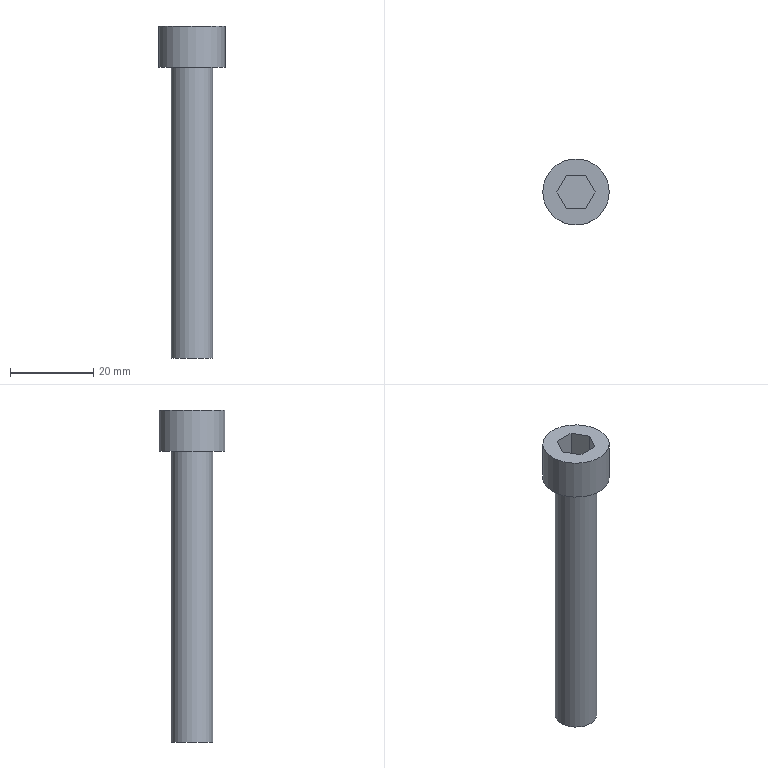Part | STEP file | 冲床-300配套压波_id14_x_t | 1 solid | 12 faces | box 16 x 16 x 80 mm | volume 7143 mm3 | plane 10 | cylinder 2 | commonest cylinder face diameters 10 x1 16 x1
STEP:
#1=CARTESIAN_POINT('',(1193.,0.,-1.));
#2=VERTEX_POINT('',#1);
#3=CARTESIAN_POINT('',(1185.,0.,-1.));
#4=DIRECTION('',(0.,0.,1.));
#5=DIRECTION('',(1.,0.,0.));
#6=AXIS2_PLACEMENT_3D('',#3,#4,#5);
#7=CIRCLE('',#6,8.);
#8=EDGE_CURVE('',#2,#2,#7,.T.);
#9=ORIENTED_EDGE('',*,*,#8,.T.);
#10=EDGE_LOOP('',(#9));
#11=FACE_BOUND('',#10,.T.);
#12=CARTESIAN_POINT('',(1182.691,4.,-1.));
#13=VERTEX_POINT('',#12);
#14=CARTESIAN_POINT('',(1187.309,4.,-1.));
#15=VERTEX_POINT('',#14);
#16=CARTESIAN_POINT('',(1182.691,4.,-1.));
#17=DIRECTION('',(1.,0.,0.));
#18=VECTOR('',#17,1.);
#19=LINE('',#16,#18);
#20=EDGE_CURVE('',#13,#15,#19,.T.);
#21=ORIENTED_EDGE('',*,*,#20,.T.);
#22=CARTESIAN_POINT('',(1189.619,0.,-1.));
#23=VERTEX_POINT('',#22);
#24=CARTESIAN_POINT('',(1187.309,4.,-1.));
#25=DIRECTION('',(0.5,-0.866,0.));
#26=VECTOR('',#25,1.);
#27=LINE('',#24,#26);
#28=EDGE_CURVE('',#15,#23,#27,.T.);
#29=ORIENTED_EDGE('',*,*,#28,.T.);
#30=CARTESIAN_POINT('',(1187.309,-4.,-1.));
#31=VERTEX_POINT('',#30);
#32=CARTESIAN_POINT('',(1189.619,0.,-1.));
#33=DIRECTION('',(-0.5,-0.866,0.));
#34=VECTOR('',#33,1.);
#35=LINE('',#32,#34);
#36=EDGE_CURVE('',#23,#31,#35,.T.);
#37=ORIENTED_EDGE('',*,*,#36,.T.);
#38=CARTESIAN_POINT('',(1182.691,-4.,-1.));
#39=VERTEX_POINT('',#38);
#40=CARTESIAN_POINT('',(1187.309,-4.,-1.));
#41=DIRECTION('',(-1.,0.,0.));
#42=VECTOR('',#41,1.);
#43=LINE('',#40,#42);
#44=EDGE_CURVE('',#31,#39,#43,.T.);
#45=ORIENTED_EDGE('',*,*,#44,.T.);
#46=CARTESIAN_POINT('',(1180.381,0.,-1.));
#47=VERTEX_POINT('',#46);
#48=CARTESIAN_POINT('',(1182.691,-4.,-1.));
#49=DIRECTION('',(-0.5,0.866,0.));
#50=VECTOR('',#49,1.);
#51=LINE('',#48,#50);
#52=EDGE_CURVE('',#39,#47,#51,.T.);
#53=ORIENTED_EDGE('',*,*,#52,.T.);
#54=CARTESIAN_POINT('',(1180.381,0.,-1.));
#55=DIRECTION('',(0.5,0.866,0.));
#56=VECTOR('',#55,1.);
#57=LINE('',#54,#56);
#58=EDGE_CURVE('',#47,#13,#57,.T.);
#59=ORIENTED_EDGE('',*,*,#58,.T.);
#60=EDGE_LOOP('',(#21,#29,#37,#45,#53,#59));
#61=FACE_BOUND('',#60,.T.);
#62=CARTESIAN_POINT('',(1193.,0.,-1.));
#63=DIRECTION('',(0.,0.,-1.));
#64=DIRECTION('',(-1.,0.,0.));
#65=AXIS2_PLACEMENT_3D('',#62,#63,#64);
#66=PLANE('',#65);
#67=ADVANCED_FACE('',(#11,#61),#66,.F.);
#68=ORIENTED_EDGE('',*,*,#8,.F.);
#69=EDGE_LOOP('',(#68));
#70=FACE_BOUND('',#69,.T.);
#71=CARTESIAN_POINT('',(1193.,0.,-11.));
#72=VERTEX_POINT('',#71);
#73=CARTESIAN_POINT('',(1185.,0.,-11.));
#74=DIRECTION('',(0.,0.,1.));
#75=DIRECTION('',(1.,0.,0.));
#76=AXIS2_PLACEMENT_3D('',#73,#74,#75);
#77=CIRCLE('',#76,8.);
#78=EDGE_CURVE('',#72,#72,#77,.T.);
#79=ORIENTED_EDGE('',*,*,#78,.T.);
#80=EDGE_LOOP('',(#79));
#81=FACE_BOUND('',#80,.T.);
#82=CARTESIAN_POINT('',(1185.,0.,-9.9));
#83=DIRECTION('',(0.,0.,1.));
#84=DIRECTION('',(1.,0.,0.));
#85=AXIS2_PLACEMENT_3D('',#82,#83,#84);
#86=CYLINDRICAL_SURFACE('',#85,8.);
#87=ADVANCED_FACE('',(#70,#81),#86,.T.);
#88=ORIENTED_EDGE('',*,*,#78,.F.);
#89=EDGE_LOOP('',(#88));
#90=FACE_BOUND('',#89,.T.);
#91=CARTESIAN_POINT('',(1190.,0.,-11.));
#92=VERTEX_POINT('',#91);
#93=CARTESIAN_POINT('',(1185.,0.,-11.));
#94=DIRECTION('',(0.,0.,1.));
#95=DIRECTION('',(1.,0.,0.));
#96=AXIS2_PLACEMENT_3D('',#93,#94,#95);
#97=CIRCLE('',#96,5.);
#98=EDGE_CURVE('',#92,#92,#97,.T.);
#99=ORIENTED_EDGE('',*,*,#98,.T.);
#100=EDGE_LOOP('',(#99));
#101=FACE_BOUND('',#100,.T.);
#102=CARTESIAN_POINT('',(1190.,0.,-11.));
#103=DIRECTION('',(0.,0.,1.));
#104=DIRECTION('',(1.,0.,0.));
#105=AXIS2_PLACEMENT_3D('',#102,#103,#104);
#106=PLANE('',#105);
#107=ADVANCED_FACE('',(#90,#101),#106,.F.);
#108=ORIENTED_EDGE('',*,*,#98,.F.);
#109=EDGE_LOOP('',(#108));
#110=FACE_BOUND('',#109,.T.);
#111=CARTESIAN_POINT('',(1190.,0.,-81.));
#112=VERTEX_POINT('',#111);
#113=CARTESIAN_POINT('',(1185.,0.,-81.));
#114=DIRECTION('',(0.,0.,1.));
#115=DIRECTION('',(1.,0.,0.));
#116=AXIS2_PLACEMENT_3D('',#113,#114,#115);
#117=CIRCLE('',#116,5.);
#118=EDGE_CURVE('',#112,#112,#117,.T.);
#119=ORIENTED_EDGE('',*,*,#118,.T.);
#120=EDGE_LOOP('',(#119));
#121=FACE_BOUND('',#120,.T.);
#122=CARTESIAN_POINT('',(1185.,0.,-9.9));
#123=DIRECTION('',(0.,0.,1.));
#124=DIRECTION('',(1.,0.,0.));
#125=AXIS2_PLACEMENT_3D('',#122,#123,#124);
#126=CYLINDRICAL_SURFACE('',#125,5.);
#127=ADVANCED_FACE('',(#110,#121),#126,.T.);
#128=ORIENTED_EDGE('',*,*,#118,.F.);
#129=EDGE_LOOP('',(#128));
#130=FACE_OUTER_BOUND('',#129,.T.);
#131=CARTESIAN_POINT('',(1185.,0.,-81.));
#132=DIRECTION('',(0.,0.,1.));
#133=DIRECTION('',(1.,0.,0.));
#134=AXIS2_PLACEMENT_3D('',#131,#132,#133);
#135=PLANE('',#134);
#136=ADVANCED_FACE('',(#130),#135,.F.);
#137=ORIENTED_EDGE('',*,*,#20,.F.);
#138=CARTESIAN_POINT('',(1182.691,4.,-7.6));
#139=VERTEX_POINT('',#138);
#140=CARTESIAN_POINT('',(1182.691,4.,-7.6));
#141=DIRECTION('',(0.,0.,-1.));
#142=VECTOR('',#141,1.);
#143=LINE('',#140,#142);
#144=EDGE_CURVE('',#13,#139,#143,.T.);
#145=ORIENTED_EDGE('',*,*,#144,.T.);
#146=CARTESIAN_POINT('',(1187.309,4.,-7.6));
#147=VERTEX_POINT('',#146);
#148=CARTESIAN_POINT('',(1182.691,4.,-7.6));
#149=DIRECTION('',(-1.,0.,0.));
#150=VECTOR('',#149,1.);
#151=LINE('',#148,#150);
#152=EDGE_CURVE('',#147,#139,#151,.T.);
#153=ORIENTED_EDGE('',*,*,#152,.F.);
#154=CARTESIAN_POINT('',(1187.309,4.,-7.6));
#155=DIRECTION('',(0.,0.,-1.));
#156=VECTOR('',#155,1.);
#157=LINE('',#154,#156);
#158=EDGE_CURVE('',#15,#147,#157,.T.);
#159=ORIENTED_EDGE('',*,*,#158,.F.);
#160=EDGE_LOOP('',(#137,#145,#153,#159));
#161=FACE_OUTER_BOUND('',#160,.T.);
#162=CARTESIAN_POINT('',(1182.691,4.,-7.6));
#163=DIRECTION('',(0.,-1.,0.));
#164=DIRECTION('',(1.,0.,0.));
#165=AXIS2_PLACEMENT_3D('',#162,#163,#164);
#166=PLANE('',#165);
#167=ADVANCED_FACE('',(#161),#166,.T.);
#168=ORIENTED_EDGE('',*,*,#28,.F.);
#169=ORIENTED_EDGE('',*,*,#158,.T.);
#170=CARTESIAN_POINT('',(1189.619,0.,-7.6));
#171=VERTEX_POINT('',#170);
#172=CARTESIAN_POINT('',(1187.309,4.,-7.6));
#173=DIRECTION('',(-0.5,0.866,0.));
#174=VECTOR('',#173,1.);
#175=LINE('',#172,#174);
#176=EDGE_CURVE('',#171,#147,#175,.T.);
#177=ORIENTED_EDGE('',*,*,#176,.F.);
#178=CARTESIAN_POINT('',(1189.619,0.,-7.6));
#179=DIRECTION('',(0.,0.,-1.));
#180=VECTOR('',#179,1.);
#181=LINE('',#178,#180);
#182=EDGE_CURVE('',#23,#171,#181,.T.);
#183=ORIENTED_EDGE('',*,*,#182,.F.);
#184=EDGE_LOOP('',(#168,#169,#177,#183));
#185=FACE_OUTER_BOUND('',#184,.T.);
#186=CARTESIAN_POINT('',(1187.309,4.,-7.6));
#187=DIRECTION('',(-0.866,-0.5,0.));
#188=DIRECTION('',(0.5,-0.866,0.));
#189=AXIS2_PLACEMENT_3D('',#186,#187,#188);
#190=PLANE('',#189);
#191=ADVANCED_FACE('',(#185),#190,.T.);
#192=ORIENTED_EDGE('',*,*,#36,.F.);
#193=ORIENTED_EDGE('',*,*,#182,.T.);
#194=CARTESIAN_POINT('',(1187.309,-4.,-7.6));
#195=VERTEX_POINT('',#194);
#196=CARTESIAN_POINT('',(1189.619,0.,-7.6));
#197=DIRECTION('',(0.5,0.866,0.));
#198=VECTOR('',#197,1.);
#199=LINE('',#196,#198);
#200=EDGE_CURVE('',#195,#171,#199,.T.);
#201=ORIENTED_EDGE('',*,*,#200,.F.);
#202=CARTESIAN_POINT('',(1187.309,-4.,-7.6));
#203=DIRECTION('',(0.,0.,-1.));
#204=VECTOR('',#203,1.);
#205=LINE('',#202,#204);
#206=EDGE_CURVE('',#31,#195,#205,.T.);
#207=ORIENTED_EDGE('',*,*,#206,.F.);
#208=EDGE_LOOP('',(#192,#193,#201,#207));
#209=FACE_OUTER_BOUND('',#208,.T.);
#210=CARTESIAN_POINT('',(1189.619,0.,-7.6));
#211=DIRECTION('',(-0.866,0.5,0.));
#212=DIRECTION('',(-0.5,-0.866,0.));
#213=AXIS2_PLACEMENT_3D('',#210,#211,#212);
#214=PLANE('',#213);
#215=ADVANCED_FACE('',(#209),#214,.T.);
#216=ORIENTED_EDGE('',*,*,#44,.F.);
#217=ORIENTED_EDGE('',*,*,#206,.T.);
#218=CARTESIAN_POINT('',(1182.691,-4.,-7.6));
#219=VERTEX_POINT('',#218);
#220=CARTESIAN_POINT('',(1187.309,-4.,-7.6));
#221=DIRECTION('',(1.,0.,0.));
#222=VECTOR('',#221,1.);
#223=LINE('',#220,#222);
#224=EDGE_CURVE('',#219,#195,#223,.T.);
#225=ORIENTED_EDGE('',*,*,#224,.F.);
#226=CARTESIAN_POINT('',(1182.691,-4.,-7.6));
#227=DIRECTION('',(0.,0.,-1.));
#228=VECTOR('',#227,1.);
#229=LINE('',#226,#228);
#230=EDGE_CURVE('',#39,#219,#229,.T.);
#231=ORIENTED_EDGE('',*,*,#230,.F.);
#232=EDGE_LOOP('',(#216,#217,#225,#231));
#233=FACE_OUTER_BOUND('',#232,.T.);
#234=CARTESIAN_POINT('',(1187.309,-4.,-7.6));
#235=DIRECTION('',(0.,1.,0.));
#236=DIRECTION('',(0.,0.,1.));
#237=AXIS2_PLACEMENT_3D('',#234,#235,#236);
#238=PLANE('',#237);
#239=ADVANCED_FACE('',(#233),#238,.T.);
#240=ORIENTED_EDGE('',*,*,#52,.F.);
#241=ORIENTED_EDGE('',*,*,#230,.T.);
#242=CARTESIAN_POINT('',(1180.381,0.,-7.6));
#243=VERTEX_POINT('',#242);
#244=CARTESIAN_POINT('',(1182.691,-4.,-7.6));
#245=DIRECTION('',(0.5,-0.866,0.));
#246=VECTOR('',#245,1.);
#247=LINE('',#244,#246);
#248=EDGE_CURVE('',#243,#219,#247,.T.);
#249=ORIENTED_EDGE('',*,*,#248,.F.);
#250=CARTESIAN_POINT('',(1180.381,0.,-7.6));
#251=DIRECTION('',(0.,0.,-1.));
#252=VECTOR('',#251,1.);
#253=LINE('',#250,#252);
#254=EDGE_CURVE('',#47,#243,#253,.T.);
#255=ORIENTED_EDGE('',*,*,#254,.F.);
#256=EDGE_LOOP('',(#240,#241,#249,#255));
#257=FACE_OUTER_BOUND('',#256,.T.);
#258=CARTESIAN_POINT('',(1182.691,-4.,-7.6));
#259=DIRECTION('',(0.866,0.5,0.));
#260=DIRECTION('',(-0.5,0.866,0.));
#261=AXIS2_PLACEMENT_3D('',#258,#259,#260);
#262=PLANE('',#261);
#263=ADVANCED_FACE('',(#257),#262,.T.);
#264=ORIENTED_EDGE('',*,*,#58,.F.);
#265=ORIENTED_EDGE('',*,*,#254,.T.);
#266=CARTESIAN_POINT('',(1180.381,0.,-7.6));
#267=DIRECTION('',(-0.5,-0.866,0.));
#268=VECTOR('',#267,1.);
#269=LINE('',#266,#268);
#270=EDGE_CURVE('',#139,#243,#269,.T.);
#271=ORIENTED_EDGE('',*,*,#270,.F.);
#272=ORIENTED_EDGE('',*,*,#144,.F.);
#273=EDGE_LOOP('',(#264,#265,#271,#272));
#274=FACE_OUTER_BOUND('',#273,.T.);
#275=CARTESIAN_POINT('',(1180.381,0.,-7.6));
#276=DIRECTION('',(0.866,-0.5,0.));
#277=DIRECTION('',(0.5,0.866,0.));
#278=AXIS2_PLACEMENT_3D('',#275,#276,#277);
#279=PLANE('',#278);
#280=ADVANCED_FACE('',(#274),#279,.T.);
#281=ORIENTED_EDGE('',*,*,#152,.T.);
#282=ORIENTED_EDGE('',*,*,#270,.T.);
#283=ORIENTED_EDGE('',*,*,#248,.T.);
#284=ORIENTED_EDGE('',*,*,#224,.T.);
#285=ORIENTED_EDGE('',*,*,#200,.T.);
#286=ORIENTED_EDGE('',*,*,#176,.T.);
#287=EDGE_LOOP('',(#281,#282,#283,#284,#285,#286));
#288=FACE_OUTER_BOUND('',#287,.T.);
#289=CARTESIAN_POINT('',(1185.,0.,-7.6));
#290=DIRECTION('',(0.,0.,-1.));
#291=DIRECTION('',(-1.,0.,0.));
#292=AXIS2_PLACEMENT_3D('',#289,#290,#291);
#293=PLANE('',#292);
#294=ADVANCED_FACE('',(#288),#293,.F.);
#295=CLOSED_SHELL('',(#67,#87,#107,#127,#136,#167,#191,#215,#239,#263,#280,#294));
#296=MANIFOLD_SOLID_BREP('',#295);
#297=(LENGTH_UNIT()NAMED_UNIT(*)SI_UNIT(.MILLI.,.METRE.));
#298=UNCERTAINTY_MEASURE_WITH_UNIT(LENGTH_MEASURE(0.00002),#297,'','');
#299=(NAMED_UNIT(*)PLANE_ANGLE_UNIT()SI_UNIT($,.RADIAN.));
#300=PLANE_ANGLE_MEASURE_WITH_UNIT(PLANE_ANGLE_MEASURE(0.01745),#299);
#301=DIMENSIONAL_EXPONENTS(0.,0.,0.,0.,0.,0.,0.);
#302=(CONVERSION_BASED_UNIT('DEGREE',#300)NAMED_UNIT(#301)PLANE_ANGLE_UNIT());
#303=(NAMED_UNIT(*)SI_UNIT($,.STERADIAN.)SOLID_ANGLE_UNIT());
#304=(GEOMETRIC_REPRESENTATION_CONTEXT(3)GLOBAL_UNCERTAINTY_ASSIGNED_CONTEXT((#298))GLOBAL_UNIT_ASSIGNED_CONTEXT((#297,#302,#303))REPRESENTATION_CONTEXT('',''));
#305=ADVANCED_BREP_SHAPE_REPRESENTATION('',(#296),#304);